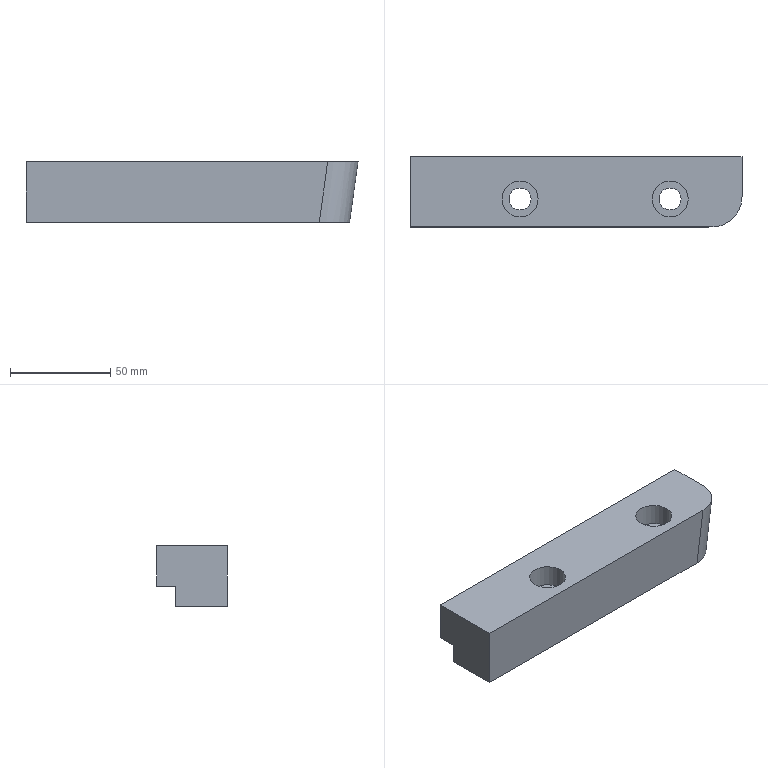Part | STEP file | solid 88 | 1 solid | 15 faces | box 165.903 x 35 x 30 mm | volume 145884 mm3 | plane 6 | cylinder 5 | spline 4 | commonest cylinder face diameters 11 x2 18 x2 30 x1